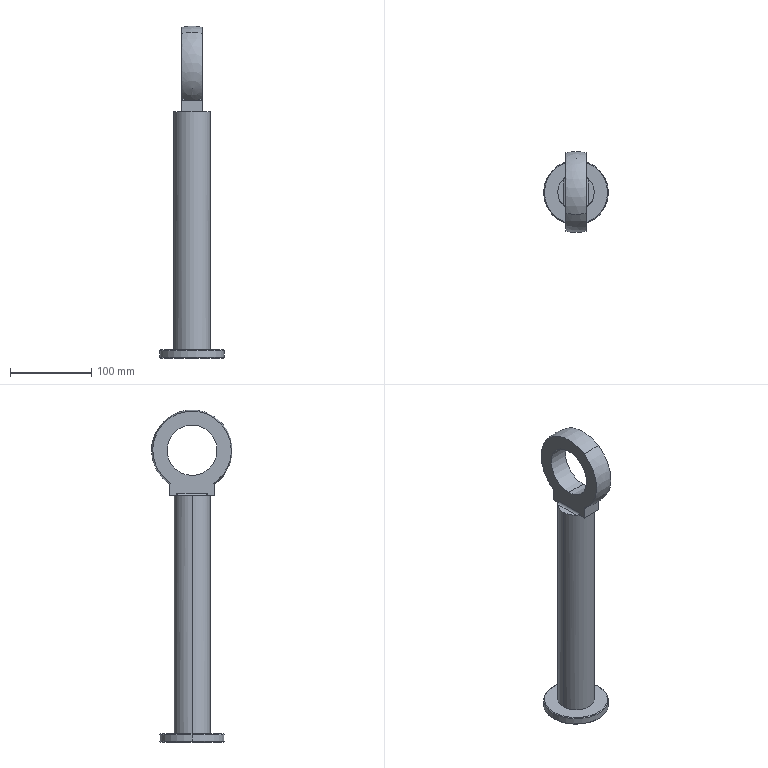Part | SolidWorks | features ICE 3, Chamfer 1, Extrusion 1, Fillet 1, RevCut 1 | 1 solid | 26 faces | box 80 x 100 x 410 mm | volume 647180 mm3 | plane 12 | cylinder 8 | cone 4 | sphere 2 | commonest cylinder face diameters 6 x2 45 x2 62 x2 80 x2
STEP:
#1=CARTESIAN_POINT('',(-12.5,0.,391.));
#2=VERTEX_POINT('',#1);
#3=CARTESIAN_POINT('',(-12.5,0.,329.));
#4=VERTEX_POINT('',#3);
#5=CARTESIAN_POINT('',(-12.5,0.,360.));
#6=DIRECTION('',(1.,0.,0.));
#7=DIRECTION('',(0.,0.,-1.));
#8=AXIS2_PLACEMENT_3D('',#5,#6,#7);
#9=CIRCLE('',#8,31.);
#10=EDGE_CURVE('',#2,#4,#9,.T.);
#11=ORIENTED_EDGE('',*,*,#10,.F.);
#12=CARTESIAN_POINT('',(12.5,0.,391.));
#13=VERTEX_POINT('',#12);
#14=CARTESIAN_POINT('',(-40.,0.,391.));
#15=DIRECTION('',(1.,0.,0.));
#16=VECTOR('',#15,1000.);
#17=LINE('',#14,#16);
#18=EDGE_CURVE('',#2,#13,#17,.T.);
#19=ORIENTED_EDGE('',*,*,#18,.T.);
#20=CARTESIAN_POINT('',(12.5,0.,329.));
#21=VERTEX_POINT('',#20);
#22=CARTESIAN_POINT('',(12.5,0.,360.));
#23=DIRECTION('',(1.,0.,0.));
#24=DIRECTION('',(0.,0.,-1.));
#25=AXIS2_PLACEMENT_3D('',#22,#23,#24);
#26=CIRCLE('',#25,31.);
#27=EDGE_CURVE('',#13,#21,#26,.T.);
#28=ORIENTED_EDGE('',*,*,#27,.T.);
#29=CARTESIAN_POINT('',(-40.,0.,329.));
#30=DIRECTION('',(1.,0.,0.));
#31=VECTOR('',#30,1000.);
#32=LINE('',#29,#31);
#33=EDGE_CURVE('',#4,#21,#32,.T.);
#34=ORIENTED_EDGE('',*,*,#33,.F.);
#35=EDGE_LOOP('',(#11,#19,#28,#34));
#36=FACE_OUTER_BOUND('',#35,.T.);
#37=CARTESIAN_POINT('',(-40.,0.,360.));
#38=DIRECTION('',(1.,0.,0.));
#39=DIRECTION('',(0.,0.,-1.));
#40=AXIS2_PLACEMENT_3D('',#37,#38,#39);
#41=CYLINDRICAL_SURFACE('',#40,31.);
#42=ADVANCED_FACE('',(#36),#41,.F.);
#43=CARTESIAN_POINT('',(-12.5,26.615,319.56));
#44=VERTEX_POINT('',#43);
#45=CARTESIAN_POINT('',(-12.5,-26.615,400.44));
#46=VERTEX_POINT('',#45);
#47=CARTESIAN_POINT('',(-12.5,0.,360.));
#48=DIRECTION('',(1.,0.,0.));
#49=DIRECTION('',(0.,0.,-1.));
#50=AXIS2_PLACEMENT_3D('',#47,#48,#49);
#51=CIRCLE('',#50,48.412);
#52=EDGE_CURVE('',#44,#46,#51,.T.);
#53=ORIENTED_EDGE('',*,*,#52,.T.);
#54=CARTESIAN_POINT('',(12.5,-26.615,400.44));
#55=VERTEX_POINT('',#54);
#56=CARTESIAN_POINT('',(0.,0.,360.));
#57=DIRECTION('',(0.,0.8353,0.5498));
#58=DIRECTION('',(0.,-0.5498,0.8353));
#59=AXIS2_PLACEMENT_3D('',#56,#57,#58);
#60=CIRCLE('',#59,50.);
#61=EDGE_CURVE('',#46,#55,#60,.T.);
#62=ORIENTED_EDGE('',*,*,#61,.T.);
#63=CARTESIAN_POINT('',(12.5,26.615,319.56));
#64=VERTEX_POINT('',#63);
#65=CARTESIAN_POINT('',(12.5,0.,360.));
#66=DIRECTION('',(1.,0.,0.));
#67=DIRECTION('',(0.,0.,-1.));
#68=AXIS2_PLACEMENT_3D('',#65,#66,#67);
#69=CIRCLE('',#68,48.412);
#70=EDGE_CURVE('',#64,#55,#69,.T.);
#71=ORIENTED_EDGE('',*,*,#70,.F.);
#72=CARTESIAN_POINT('',(0.,0.,360.));
#73=DIRECTION('',(0.,0.8353,0.5498));
#74=DIRECTION('',(0.,0.5498,-0.8353));
#75=AXIS2_PLACEMENT_3D('',#72,#73,#74);
#76=CIRCLE('',#75,50.);
#77=EDGE_CURVE('',#64,#44,#76,.T.);
#78=ORIENTED_EDGE('',*,*,#77,.T.);
#79=EDGE_LOOP('',(#53,#62,#71,#78));
#80=FACE_OUTER_BOUND('',#79,.T.);
#81=CARTESIAN_POINT('',(0.,0.,360.));
#82=DIRECTION('',(0.,0.8353,0.5498));
#83=DIRECTION('',(0.,0.5498,-0.8353));
#84=AXIS2_PLACEMENT_3D('',#81,#82,#83);
#85=SPHERICAL_SURFACE('',#84,50.);
#86=ADVANCED_FACE('',(#80),#85,.T.);
#87=CARTESIAN_POINT('',(39.,0.,10.));
#88=VERTEX_POINT('',#87);
#89=CARTESIAN_POINT('',(-39.,0.,10.));
#90=VERTEX_POINT('',#89);
#91=CARTESIAN_POINT('',(0.,0.,10.));
#92=DIRECTION('',(0.,0.,1.));
#93=DIRECTION('',(1.,0.,0.));
#94=AXIS2_PLACEMENT_3D('',#91,#92,#93);
#95=CIRCLE('',#94,39.);
#96=EDGE_CURVE('',#88,#90,#95,.T.);
#97=ORIENTED_EDGE('',*,*,#96,.F.);
#98=CARTESIAN_POINT('',(40.,0.,9.));
#99=VERTEX_POINT('',#98);
#100=CARTESIAN_POINT('',(39.,0.,10.));
#101=DIRECTION('',(0.7071,0.,-0.7071));
#102=VECTOR('',#101,1000.);
#103=LINE('',#100,#102);
#104=EDGE_CURVE('',#88,#99,#103,.T.);
#105=ORIENTED_EDGE('',*,*,#104,.T.);
#106=CARTESIAN_POINT('',(-40.,0.,9.));
#107=VERTEX_POINT('',#106);
#108=CARTESIAN_POINT('',(0.,0.,9.));
#109=DIRECTION('',(0.,0.,-1.));
#110=DIRECTION('',(1.,0.,0.));
#111=AXIS2_PLACEMENT_3D('',#108,#109,#110);
#112=CIRCLE('',#111,40.);
#113=EDGE_CURVE('',#107,#99,#112,.T.);
#114=ORIENTED_EDGE('',*,*,#113,.F.);
#115=CARTESIAN_POINT('',(-39.,0.,10.));
#116=DIRECTION('',(-0.7071,0.,-0.7071));
#117=VECTOR('',#116,1000.);
#118=LINE('',#115,#117);
#119=EDGE_CURVE('',#90,#107,#118,.T.);
#120=ORIENTED_EDGE('',*,*,#119,.F.);
#121=EDGE_LOOP('',(#97,#105,#114,#120));
#122=FACE_OUTER_BOUND('',#121,.T.);
#123=CARTESIAN_POINT('',(0.,0.,10.));
#124=DIRECTION('',(0.,0.,-1.));
#125=DIRECTION('',(-1.,0.,0.));
#126=AXIS2_PLACEMENT_3D('',#123,#124,#125);
#127=CONICAL_SURFACE('',#126,39.,0.7854);
#128=ADVANCED_FACE('',(#122),#127,.T.);
#129=CARTESIAN_POINT('',(-39.,0.,0.));
#130=VERTEX_POINT('',#129);
#131=CARTESIAN_POINT('',(39.,0.,0.));
#132=VERTEX_POINT('',#131);
#133=CARTESIAN_POINT('',(0.,0.,0.));
#134=DIRECTION('',(0.,0.,-1.));
#135=DIRECTION('',(1.,0.,0.));
#136=AXIS2_PLACEMENT_3D('',#133,#134,#135);
#137=CIRCLE('',#136,39.);
#138=EDGE_CURVE('',#130,#132,#137,.T.);
#139=ORIENTED_EDGE('',*,*,#138,.F.);
#140=CARTESIAN_POINT('',(-40.,0.,1.));
#141=VERTEX_POINT('',#140);
#142=CARTESIAN_POINT('',(-40.,0.,1.));
#143=DIRECTION('',(-0.7071,0.,0.7071));
#144=VECTOR('',#143,1000.);
#145=LINE('',#142,#144);
#146=EDGE_CURVE('',#130,#141,#145,.T.);
#147=ORIENTED_EDGE('',*,*,#146,.T.);
#148=CARTESIAN_POINT('',(40.,0.,1.));
#149=VERTEX_POINT('',#148);
#150=CARTESIAN_POINT('',(0.,0.,1.));
#151=DIRECTION('',(0.,0.,1.));
#152=DIRECTION('',(1.,0.,0.));
#153=AXIS2_PLACEMENT_3D('',#150,#151,#152);
#154=CIRCLE('',#153,40.);
#155=EDGE_CURVE('',#149,#141,#154,.T.);
#156=ORIENTED_EDGE('',*,*,#155,.F.);
#157=CARTESIAN_POINT('',(40.,0.,1.));
#158=DIRECTION('',(0.7071,0.,0.7071));
#159=VECTOR('',#158,1000.);
#160=LINE('',#157,#159);
#161=EDGE_CURVE('',#132,#149,#160,.T.);
#162=ORIENTED_EDGE('',*,*,#161,.F.);
#163=EDGE_LOOP('',(#139,#147,#156,#162));
#164=FACE_OUTER_BOUND('',#163,.T.);
#165=CARTESIAN_POINT('',(0.,0.,1.));
#166=DIRECTION('',(0.,0.,1.));
#167=DIRECTION('',(1.,0.,0.));
#168=AXIS2_PLACEMENT_3D('',#165,#166,#167);
#169=CONICAL_SURFACE('',#168,40.,0.7854);
#170=ADVANCED_FACE('',(#164),#169,.T.);
#171=CARTESIAN_POINT('',(22.5,0.,304.));
#172=VERTEX_POINT('',#171);
#173=CARTESIAN_POINT('',(15.5,16.31,304.));
#174=VERTEX_POINT('',#173);
#175=CARTESIAN_POINT('',(0.,0.,304.));
#176=DIRECTION('',(0.,0.,1.));
#177=DIRECTION('',(1.,0.,0.));
#178=AXIS2_PLACEMENT_3D('',#175,#176,#177);
#179=CIRCLE('',#178,22.5);
#180=EDGE_CURVE('',#172,#174,#179,.T.);
#181=ORIENTED_EDGE('',*,*,#180,.F.);
#182=CARTESIAN_POINT('',(22.5,0.,10.));
#183=VERTEX_POINT('',#182);
#184=CARTESIAN_POINT('',(22.5,0.,304.));
#185=DIRECTION('',(0.,0.,-1.));
#186=VECTOR('',#185,1000.);
#187=LINE('',#184,#186);
#188=EDGE_CURVE('',#172,#183,#187,.T.);
#189=ORIENTED_EDGE('',*,*,#188,.T.);
#190=CARTESIAN_POINT('',(-22.5,0.,10.));
#191=VERTEX_POINT('',#190);
#192=CARTESIAN_POINT('',(0.,0.,10.));
#193=DIRECTION('',(0.,0.,1.));
#194=DIRECTION('',(1.,0.,0.));
#195=AXIS2_PLACEMENT_3D('',#192,#193,#194);
#196=CIRCLE('',#195,22.5);
#197=EDGE_CURVE('',#183,#191,#196,.T.);
#198=ORIENTED_EDGE('',*,*,#197,.T.);
#199=CARTESIAN_POINT('',(-22.5,0.,304.));
#200=VERTEX_POINT('',#199);
#201=CARTESIAN_POINT('',(-22.5,0.,304.));
#202=DIRECTION('',(0.,0.,-1.));
#203=VECTOR('',#202,1000.);
#204=LINE('',#201,#203);
#205=EDGE_CURVE('',#200,#191,#204,.T.);
#206=ORIENTED_EDGE('',*,*,#205,.F.);
#207=CARTESIAN_POINT('',(-15.5,16.31,304.));
#208=VERTEX_POINT('',#207);
#209=CARTESIAN_POINT('',(0.,0.,304.));
#210=DIRECTION('',(0.,0.,1.));
#211=DIRECTION('',(1.,0.,0.));
#212=AXIS2_PLACEMENT_3D('',#209,#210,#211);
#213=CIRCLE('',#212,22.5);
#214=EDGE_CURVE('',#208,#200,#213,.T.);
#215=ORIENTED_EDGE('',*,*,#214,.F.);
#216=CARTESIAN_POINT('',(-12.5,18.708,307.));
#217=VERTEX_POINT('',#216);
#218=CARTESIAN_POINT('',(-15.5,16.31,304.));
#219=CARTESIAN_POINT('',(-15.171,16.622,304.));
#220=CARTESIAN_POINT('',(-14.838,16.92,304.053));
#221=CARTESIAN_POINT('',(-14.337,17.342,304.229));
#222=CARTESIAN_POINT('',(-14.17,17.479,304.305));
#223=CARTESIAN_POINT('',(-13.849,17.734,304.488));
#224=CARTESIAN_POINT('',(-13.693,17.855,304.597));
#225=CARTESIAN_POINT('',(-13.394,18.08,304.855));
#226=CARTESIAN_POINT('',(-13.254,18.183,305.001));
#227=CARTESIAN_POINT('',(-13.001,18.364,305.327));
#228=CARTESIAN_POINT('',(-12.887,18.444,305.511));
#229=CARTESIAN_POINT('',(-12.701,18.573,305.9));
#230=CARTESIAN_POINT('',(-12.627,18.623,306.106));
#231=CARTESIAN_POINT('',(-12.526,18.691,306.544));
#232=CARTESIAN_POINT('',(-12.5,18.708,306.771));
#233=CARTESIAN_POINT('',(-12.5,18.708,307.));
#234=B_SPLINE_CURVE_WITH_KNOTS('',3,(#218,#219,#220,#221,#222,#223,#224,#225,#226,#227,#228,#229,#230,#231,#232,#233),.UNSPECIFIED.,.F.,.F.,(4,2,2,2,2,2,2,4),(0.,0.001348,0.002022,0.002696,0.003369,0.004043,0.004717,0.005391),.UNSPECIFIED.);
#235=EDGE_CURVE('',#208,#217,#234,.T.);
#236=ORIENTED_EDGE('',*,*,#235,.T.);
#237=CARTESIAN_POINT('',(-12.5,18.708,304.));
#238=VERTEX_POINT('',#237);
#239=CARTESIAN_POINT('',(-12.5,18.708,304.));
#240=DIRECTION('',(0.,0.,1.));
#241=VECTOR('',#240,1000.);
#242=LINE('',#239,#241);
#243=EDGE_CURVE('',#238,#217,#242,.T.);
#244=ORIENTED_EDGE('',*,*,#243,.F.);
#245=CARTESIAN_POINT('',(12.5,18.708,304.));
#246=VERTEX_POINT('',#245);
#247=CARTESIAN_POINT('',(0.,0.,304.));
#248=DIRECTION('',(0.,0.,1.));
#249=DIRECTION('',(1.,0.,0.));
#250=AXIS2_PLACEMENT_3D('',#247,#248,#249);
#251=CIRCLE('',#250,22.5);
#252=EDGE_CURVE('',#246,#238,#251,.T.);
#253=ORIENTED_EDGE('',*,*,#252,.F.);
#254=CARTESIAN_POINT('',(12.5,18.708,307.));
#255=VERTEX_POINT('',#254);
#256=CARTESIAN_POINT('',(12.5,18.708,307.));
#257=DIRECTION('',(0.,0.,-1.));
#258=VECTOR('',#257,1000.);
#259=LINE('',#256,#258);
#260=EDGE_CURVE('',#255,#246,#259,.T.);
#261=ORIENTED_EDGE('',*,*,#260,.F.);
#262=CARTESIAN_POINT('',(12.5,18.708,307.));
#263=CARTESIAN_POINT('',(12.5,18.708,306.771));
#264=CARTESIAN_POINT('',(12.526,18.691,306.548));
#265=CARTESIAN_POINT('',(12.626,18.624,306.112));
#266=CARTESIAN_POINT('',(12.7,18.573,305.901));
#267=CARTESIAN_POINT('',(12.887,18.444,305.511));
#268=CARTESIAN_POINT('',(13.001,18.365,305.328));
#269=CARTESIAN_POINT('',(13.254,18.183,305.));
#270=CARTESIAN_POINT('',(13.394,18.08,304.854));
#271=CARTESIAN_POINT('',(13.693,17.854,304.597));
#272=CARTESIAN_POINT('',(13.85,17.733,304.488));
#273=CARTESIAN_POINT('',(14.173,17.477,304.303));
#274=CARTESIAN_POINT('',(14.34,17.34,304.228));
#275=CARTESIAN_POINT('',(14.839,16.919,304.053));
#276=CARTESIAN_POINT('',(15.171,16.622,304.));
#277=CARTESIAN_POINT('',(15.5,16.31,304.));
#278=B_SPLINE_CURVE_WITH_KNOTS('',3,(#262,#263,#264,#265,#266,#267,#268,#269,#270,#271,#272,#273,#274,#275,#276,#277),.UNSPECIFIED.,.F.,.F.,(4,2,2,2,2,2,2,4),(0.,0.0006752,0.00135,0.002026,0.002701,0.003376,0.004051,0.005402),.UNSPECIFIED.);
#279=EDGE_CURVE('',#255,#174,#278,.T.);
#280=ORIENTED_EDGE('',*,*,#279,.T.);
#281=EDGE_LOOP('',(#181,#189,#198,#206,#215,#236,#244,#253,#261,#280));
#282=FACE_OUTER_BOUND('',#281,.T.);
#283=CARTESIAN_POINT('',(0.,0.,304.));
#284=DIRECTION('',(0.,0.,-1.));
#285=DIRECTION('',(-1.,0.,0.));
#286=AXIS2_PLACEMENT_3D('',#283,#284,#285);
#287=CYLINDRICAL_SURFACE('',#286,22.5);
#288=ADVANCED_FACE('',(#282),#287,.T.);
#289=ORIENTED_EDGE('',*,*,#113,.T.);
#290=CARTESIAN_POINT('',(40.,0.,10.));
#291=DIRECTION('',(0.,0.,-1.));
#292=VECTOR('',#291,1000.);
#293=LINE('',#290,#292);
#294=EDGE_CURVE('',#99,#149,#293,.T.);
#295=ORIENTED_EDGE('',*,*,#294,.T.);
#296=ORIENTED_EDGE('',*,*,#155,.T.);
#297=CARTESIAN_POINT('',(-40.,0.,10.));
#298=DIRECTION('',(0.,0.,-1.));
#299=VECTOR('',#298,1000.);
#300=LINE('',#297,#299);
#301=EDGE_CURVE('',#107,#141,#300,.T.);
#302=ORIENTED_EDGE('',*,*,#301,.F.);
#303=EDGE_LOOP('',(#289,#295,#296,#302));
#304=FACE_OUTER_BOUND('',#303,.T.);
#305=CARTESIAN_POINT('',(0.,0.,10.));
#306=DIRECTION('',(0.,0.,-1.));
#307=DIRECTION('',(-1.,0.,0.));
#308=AXIS2_PLACEMENT_3D('',#305,#306,#307);
#309=CYLINDRICAL_SURFACE('',#308,40.);
#310=ADVANCED_FACE('',(#304),#309,.T.);
#311=CARTESIAN_POINT('',(-12.5,-27.5,318.215));
#312=VERTEX_POINT('',#311);
#313=CARTESIAN_POINT('',(12.5,-27.5,318.215));
#314=VERTEX_POINT('',#313);
#315=CARTESIAN_POINT('',(12.5,-27.5,318.215));
#316=DIRECTION('',(1.,0.,0.));
#317=VECTOR('',#316,1000.);
#318=LINE('',#315,#317);
#319=EDGE_CURVE('',#312,#314,#318,.T.);
#320=ORIENTED_EDGE('',*,*,#319,.F.);
#321=CARTESIAN_POINT('',(-12.5,-27.5,304.));
#322=VERTEX_POINT('',#321);
#323=CARTESIAN_POINT('',(-12.5,-27.5,304.));
#324=DIRECTION('',(0.,0.,-1.));
#325=VECTOR('',#324,1000.);
#326=LINE('',#323,#325);
#327=EDGE_CURVE('',#312,#322,#326,.T.);
#328=ORIENTED_EDGE('',*,*,#327,.T.);
#329=CARTESIAN_POINT('',(12.5,-27.5,304.));
#330=VERTEX_POINT('',#329);
#331=CARTESIAN_POINT('',(12.5,-27.5,304.));
#332=DIRECTION('',(-1.,0.,0.));
#333=VECTOR('',#332,1000.);
#334=LINE('',#331,#333);
#335=EDGE_CURVE('',#330,#322,#334,.T.);
#336=ORIENTED_EDGE('',*,*,#335,.F.);
#337=CARTESIAN_POINT('',(12.5,-27.5,304.));
#338=DIRECTION('',(0.,0.,-1.));
#339=VECTOR('',#338,1000.);
#340=LINE('',#337,#339);
#341=EDGE_CURVE('',#314,#330,#340,.T.);
#342=ORIENTED_EDGE('',*,*,#341,.F.);
#343=EDGE_LOOP('',(#320,#328,#336,#342));
#344=FACE_OUTER_BOUND('',#343,.T.);
#345=CARTESIAN_POINT('',(12.5,-27.5,304.));
#346=DIRECTION('',(0.,1.,0.));
#347=DIRECTION('',(0.,0.,1.));
#348=AXIS2_PLACEMENT_3D('',#345,#346,#347);
#349=PLANE('',#348);
#350=ADVANCED_FACE('',(#344),#349,.F.);
#351=ORIENTED_EDGE('',*,*,#214,.T.);
#352=CARTESIAN_POINT('',(-15.5,-16.31,304.));
#353=VERTEX_POINT('',#352);
#354=CARTESIAN_POINT('',(0.,0.,304.));
#355=DIRECTION('',(0.,0.,1.));
#356=DIRECTION('',(1.,0.,0.));
#357=AXIS2_PLACEMENT_3D('',#354,#355,#356);
#358=CIRCLE('',#357,22.5);
#359=EDGE_CURVE('',#200,#353,#358,.T.);
#360=ORIENTED_EDGE('',*,*,#359,.T.);
#361=CARTESIAN_POINT('',(-15.5,0.,304.));
#362=DIRECTION('',(0.,1.,0.));
#363=VECTOR('',#362,1000.);
#364=LINE('',#361,#363);
#365=EDGE_CURVE('',#353,#208,#364,.T.);
#366=ORIENTED_EDGE('',*,*,#365,.T.);
#367=EDGE_LOOP('',(#351,#360,#366));
#368=FACE_OUTER_BOUND('',#367,.T.);
#369=CARTESIAN_POINT('',(0.,0.,304.));
#370=DIRECTION('',(0.,0.,1.));
#371=DIRECTION('',(1.,0.,0.));
#372=AXIS2_PLACEMENT_3D('',#369,#370,#371);
#373=PLANE('',#372);
#374=ADVANCED_FACE('',(#368),#373,.T.);
#375=CARTESIAN_POINT('',(0.,0.,10.));
#376=DIRECTION('',(0.,0.,1.));
#377=DIRECTION('',(1.,0.,0.));
#378=AXIS2_PLACEMENT_3D('',#375,#376,#377);
#379=CIRCLE('',#378,39.);
#380=EDGE_CURVE('',#90,#88,#379,.T.);
#381=ORIENTED_EDGE('',*,*,#380,.T.);
#382=ORIENTED_EDGE('',*,*,#96,.T.);
#383=EDGE_LOOP('',(#381,#382));
#384=FACE_OUTER_BOUND('',#383,.T.);
#385=CARTESIAN_POINT('',(0.,0.,10.));
#386=DIRECTION('',(0.,0.,1.));
#387=DIRECTION('',(1.,0.,0.));
#388=AXIS2_PLACEMENT_3D('',#385,#386,#387);
#389=CIRCLE('',#388,22.5);
#390=EDGE_CURVE('',#191,#183,#389,.T.);
#391=ORIENTED_EDGE('',*,*,#390,.F.);
#392=ORIENTED_EDGE('',*,*,#197,.F.);
#393=EDGE_LOOP('',(#391,#392));
#394=FACE_BOUND('',#393,.T.);
#395=CARTESIAN_POINT('',(0.,0.,10.));
#396=DIRECTION('',(0.,0.,1.));
#397=DIRECTION('',(1.,0.,0.));
#398=AXIS2_PLACEMENT_3D('',#395,#396,#397);
#399=PLANE('',#398);
#400=ADVANCED_FACE('',(#384,#394),#399,.T.);
#401=ORIENTED_EDGE('',*,*,#294,.F.);
#402=CARTESIAN_POINT('',(0.,0.,9.));
#403=DIRECTION('',(0.,0.,-1.));
#404=DIRECTION('',(1.,0.,0.));
#405=AXIS2_PLACEMENT_3D('',#402,#403,#404);
#406=CIRCLE('',#405,40.);
#407=EDGE_CURVE('',#99,#107,#406,.T.);
#408=ORIENTED_EDGE('',*,*,#407,.T.);
#409=ORIENTED_EDGE('',*,*,#301,.T.);
#410=CARTESIAN_POINT('',(0.,0.,1.));
#411=DIRECTION('',(0.,0.,1.));
#412=DIRECTION('',(1.,0.,0.));
#413=AXIS2_PLACEMENT_3D('',#410,#411,#412);
#414=CIRCLE('',#413,40.);
#415=EDGE_CURVE('',#141,#149,#414,.T.);
#416=ORIENTED_EDGE('',*,*,#415,.T.);
#417=EDGE_LOOP('',(#401,#408,#409,#416));
#418=FACE_OUTER_BOUND('',#417,.T.);
#419=CARTESIAN_POINT('',(0.,0.,10.));
#420=DIRECTION('',(0.,0.,-1.));
#421=DIRECTION('',(-1.,0.,0.));
#422=AXIS2_PLACEMENT_3D('',#419,#420,#421);
#423=CYLINDRICAL_SURFACE('',#422,40.);
#424=ADVANCED_FACE('',(#418),#423,.T.);
#425=CARTESIAN_POINT('',(0.,0.,0.));
#426=DIRECTION('',(0.,0.,-1.));
#427=DIRECTION('',(1.,0.,0.));
#428=AXIS2_PLACEMENT_3D('',#425,#426,#427);
#429=CIRCLE('',#428,39.);
#430=EDGE_CURVE('',#132,#130,#429,.T.);
#431=ORIENTED_EDGE('',*,*,#430,.T.);
#432=ORIENTED_EDGE('',*,*,#138,.T.);
#433=EDGE_LOOP('',(#431,#432));
#434=FACE_OUTER_BOUND('',#433,.T.);
#435=CARTESIAN_POINT('',(0.,0.,0.));
#436=DIRECTION('',(0.,0.,1.));
#437=DIRECTION('',(1.,0.,0.));
#438=AXIS2_PLACEMENT_3D('',#435,#436,#437);
#439=PLANE('',#438);
#440=ADVANCED_FACE('',(#434),#439,.F.);
#441=ORIENTED_EDGE('',*,*,#188,.F.);
#442=CARTESIAN_POINT('',(15.5,-16.31,304.));
#443=VERTEX_POINT('',#442);
#444=CARTESIAN_POINT('',(0.,0.,304.));
#445=DIRECTION('',(0.,0.,1.));
#446=DIRECTION('',(1.,0.,0.));
#447=AXIS2_PLACEMENT_3D('',#444,#445,#446);
#448=CIRCLE('',#447,22.5);
#449=EDGE_CURVE('',#443,#172,#448,.T.);
#450=ORIENTED_EDGE('',*,*,#449,.F.);
#451=CARTESIAN_POINT('',(12.5,-18.708,307.));
#452=VERTEX_POINT('',#451);
#453=CARTESIAN_POINT('',(15.5,-16.31,304.));
#454=CARTESIAN_POINT('',(15.171,-16.622,304.));
#455=CARTESIAN_POINT('',(14.838,-16.92,304.053));
#456=CARTESIAN_POINT('',(14.337,-17.342,304.229));
#457=CARTESIAN_POINT('',(14.17,-17.479,304.305));
#458=CARTESIAN_POINT('',(13.849,-17.734,304.488));
#459=CARTESIAN_POINT('',(13.693,-17.855,304.597));
#460=CARTESIAN_POINT('',(13.394,-18.08,304.855));
#461=CARTESIAN_POINT('',(13.254,-18.183,305.001));
#462=CARTESIAN_POINT('',(13.001,-18.364,305.327));
#463=CARTESIAN_POINT('',(12.887,-18.444,305.511));
#464=CARTESIAN_POINT('',(12.701,-18.573,305.9));
#465=CARTESIAN_POINT('',(12.627,-18.623,306.106));
#466=CARTESIAN_POINT('',(12.526,-18.691,306.544));
#467=CARTESIAN_POINT('',(12.5,-18.708,306.771));
#468=CARTESIAN_POINT('',(12.5,-18.708,307.));
#469=B_SPLINE_CURVE_WITH_KNOTS('',3,(#453,#454,#455,#456,#457,#458,#459,#460,#461,#462,#463,#464,#465,#466,#467,#468),.UNSPECIFIED.,.F.,.F.,(4,2,2,2,2,2,2,4),(0.,0.001348,0.002022,0.002696,0.003369,0.004043,0.004717,0.005391),.UNSPECIFIED.);
#470=EDGE_CURVE('',#443,#452,#469,.T.);
#471=ORIENTED_EDGE('',*,*,#470,.T.);
#472=CARTESIAN_POINT('',(12.5,-18.708,304.));
#473=VERTEX_POINT('',#472);
#474=CARTESIAN_POINT('',(12.5,-18.708,304.));
#475=DIRECTION('',(0.,0.,1.));
#476=VECTOR('',#475,1000.);
#477=LINE('',#474,#476);
#478=EDGE_CURVE('',#473,#452,#477,.T.);
#479=ORIENTED_EDGE('',*,*,#478,.F.);
#480=CARTESIAN_POINT('',(-12.5,-18.708,304.));
#481=VERTEX_POINT('',#480);
#482=CARTESIAN_POINT('',(0.,0.,304.));
#483=DIRECTION('',(0.,0.,1.));
#484=DIRECTION('',(1.,0.,0.));
#485=AXIS2_PLACEMENT_3D('',#482,#483,#484);
#486=CIRCLE('',#485,22.5);
#487=EDGE_CURVE('',#481,#473,#486,.T.);
#488=ORIENTED_EDGE('',*,*,#487,.F.);
#489=CARTESIAN_POINT('',(-12.5,-18.708,307.));
#490=VERTEX_POINT('',#489);
#491=CARTESIAN_POINT('',(-12.5,-18.708,307.));
#492=DIRECTION('',(0.,0.,-1.));
#493=VECTOR('',#492,1000.);
#494=LINE('',#491,#493);
#495=EDGE_CURVE('',#490,#481,#494,.T.);
#496=ORIENTED_EDGE('',*,*,#495,.F.);
#497=CARTESIAN_POINT('',(-12.5,-18.708,307.));
#498=CARTESIAN_POINT('',(-12.5,-18.708,306.771));
#499=CARTESIAN_POINT('',(-12.526,-18.691,306.548));
#500=CARTESIAN_POINT('',(-12.626,-18.624,306.112));
#501=CARTESIAN_POINT('',(-12.7,-18.573,305.901));
#502=CARTESIAN_POINT('',(-12.887,-18.444,305.511));
#503=CARTESIAN_POINT('',(-13.001,-18.365,305.328));
#504=CARTESIAN_POINT('',(-13.254,-18.183,305.));
#505=CARTESIAN_POINT('',(-13.394,-18.08,304.854));
#506=CARTESIAN_POINT('',(-13.693,-17.854,304.597));
#507=CARTESIAN_POINT('',(-13.85,-17.733,304.488));
#508=CARTESIAN_POINT('',(-14.173,-17.477,304.303));
#509=CARTESIAN_POINT('',(-14.34,-17.34,304.228));
#510=CARTESIAN_POINT('',(-14.839,-16.919,304.053));
#511=CARTESIAN_POINT('',(-15.171,-16.622,304.));
#512=CARTESIAN_POINT('',(-15.5,-16.31,304.));
#513=B_SPLINE_CURVE_WITH_KNOTS('',3,(#497,#498,#499,#500,#501,#502,#503,#504,#505,#506,#507,#508,#509,#510,#511,#512),.UNSPECIFIED.,.F.,.F.,(4,2,2,2,2,2,2,4),(0.,0.0006752,0.00135,0.002026,0.002701,0.003376,0.004051,0.005402),.UNSPECIFIED.);
#514=EDGE_CURVE('',#490,#353,#513,.T.);
#515=ORIENTED_EDGE('',*,*,#514,.T.);
#516=ORIENTED_EDGE('',*,*,#359,.F.);
#517=ORIENTED_EDGE('',*,*,#205,.T.);
#518=ORIENTED_EDGE('',*,*,#390,.T.);
#519=EDGE_LOOP('',(#441,#450,#471,#479,#488,#496,#515,#516,#517,#518));
#520=FACE_OUTER_BOUND('',#519,.T.);
#521=CARTESIAN_POINT('',(0.,0.,304.));
#522=DIRECTION('',(0.,0.,-1.));
#523=DIRECTION('',(-1.,0.,0.));
#524=AXIS2_PLACEMENT_3D('',#521,#522,#523);
#525=CYLINDRICAL_SURFACE('',#524,22.5);
#526=ADVANCED_FACE('',(#520),#525,.T.);
#527=ORIENTED_EDGE('',*,*,#449,.T.);
#528=ORIENTED_EDGE('',*,*,#180,.T.);
#529=CARTESIAN_POINT('',(15.5,-18.708,304.));
#530=DIRECTION('',(0.,-1.,0.));
#531=VECTOR('',#530,1000.);
#532=LINE('',#529,#531);
#533=EDGE_CURVE('',#174,#443,#532,.T.);
#534=ORIENTED_EDGE('',*,*,#533,.T.);
#535=EDGE_LOOP('',(#527,#528,#534));
#536=FACE_OUTER_BOUND('',#535,.T.);
#537=CARTESIAN_POINT('',(0.,0.,304.));
#538=DIRECTION('',(0.,0.,1.));
#539=DIRECTION('',(1.,0.,0.));
#540=AXIS2_PLACEMENT_3D('',#537,#538,#539);
#541=PLANE('',#540);
#542=ADVANCED_FACE('',(#536),#541,.T.);
#543=ORIENTED_EDGE('',*,*,#146,.F.);
#544=ORIENTED_EDGE('',*,*,#430,.F.);
#545=ORIENTED_EDGE('',*,*,#161,.T.);
#546=ORIENTED_EDGE('',*,*,#415,.F.);
#547=EDGE_LOOP('',(#543,#544,#545,#546));
#548=FACE_OUTER_BOUND('',#547,.T.);
#549=CARTESIAN_POINT('',(0.,0.,1.));
#550=DIRECTION('',(0.,0.,1.));
#551=DIRECTION('',(1.,0.,0.));
#552=AXIS2_PLACEMENT_3D('',#549,#550,#551);
#553=CONICAL_SURFACE('',#552,40.,0.7854);
#554=ADVANCED_FACE('',(#548),#553,.T.);
#555=ORIENTED_EDGE('',*,*,#104,.F.);
#556=ORIENTED_EDGE('',*,*,#380,.F.);
#557=ORIENTED_EDGE('',*,*,#119,.T.);
#558=ORIENTED_EDGE('',*,*,#407,.F.);
#559=EDGE_LOOP('',(#555,#556,#557,#558));
#560=FACE_OUTER_BOUND('',#559,.T.);
#561=CARTESIAN_POINT('',(0.,0.,10.));
#562=DIRECTION('',(0.,0.,-1.));
#563=DIRECTION('',(-1.,0.,0.));
#564=AXIS2_PLACEMENT_3D('',#561,#562,#563);
#565=CONICAL_SURFACE('',#564,39.,0.7854);
#566=ADVANCED_FACE('',(#560),#565,.T.);
#567=CARTESIAN_POINT('',(12.5,27.5,304.));
#568=VERTEX_POINT('',#567);
#569=CARTESIAN_POINT('',(12.5,27.5,304.));
#570=DIRECTION('',(0.,1.,0.));
#571=VECTOR('',#570,1000.);
#572=LINE('',#569,#571);
#573=EDGE_CURVE('',#246,#568,#572,.T.);
#574=ORIENTED_EDGE('',*,*,#573,.F.);
#575=ORIENTED_EDGE('',*,*,#252,.T.);
#576=CARTESIAN_POINT('',(-12.5,27.5,304.));
#577=VERTEX_POINT('',#576);
#578=CARTESIAN_POINT('',(-12.5,27.5,304.));
#579=DIRECTION('',(0.,1.,0.));
#580=VECTOR('',#579,1000.);
#581=LINE('',#578,#580);
#582=EDGE_CURVE('',#238,#577,#581,.T.);
#583=ORIENTED_EDGE('',*,*,#582,.T.);
#584=CARTESIAN_POINT('',(12.5,27.5,304.));
#585=DIRECTION('',(-1.,0.,0.));
#586=VECTOR('',#585,1000.);
#587=LINE('',#584,#586);
#588=EDGE_CURVE('',#568,#577,#587,.T.);
#589=ORIENTED_EDGE('',*,*,#588,.F.);
#590=EDGE_LOOP('',(#574,#575,#583,#589));
#591=FACE_OUTER_BOUND('',#590,.T.);
#592=CARTESIAN_POINT('',(12.5,27.5,304.));
#593=DIRECTION('',(0.,0.,1.));
#594=DIRECTION('',(1.,0.,0.));
#595=AXIS2_PLACEMENT_3D('',#592,#593,#594);
#596=PLANE('',#595);
#597=ADVANCED_FACE('',(#591),#596,.F.);
#598=CARTESIAN_POINT('',(-12.5,27.5,304.));
#599=DIRECTION('',(0.,1.,0.));
#600=VECTOR('',#599,1000.);
#601=LINE('',#598,#600);
#602=EDGE_CURVE('',#322,#481,#601,.T.);
#603=ORIENTED_EDGE('',*,*,#602,.T.);
#604=ORIENTED_EDGE('',*,*,#487,.T.);
#605=CARTESIAN_POINT('',(12.5,27.5,304.));
#606=DIRECTION('',(0.,1.,0.));
#607=VECTOR('',#606,1000.);
#608=LINE('',#605,#607);
#609=EDGE_CURVE('',#330,#473,#608,.T.);
#610=ORIENTED_EDGE('',*,*,#609,.F.);
#611=ORIENTED_EDGE('',*,*,#335,.T.);
#612=EDGE_LOOP('',(#603,#604,#610,#611));
#613=FACE_OUTER_BOUND('',#612,.T.);
#614=CARTESIAN_POINT('',(12.5,27.5,304.));
#615=DIRECTION('',(0.,0.,1.));
#616=DIRECTION('',(1.,0.,0.));
#617=AXIS2_PLACEMENT_3D('',#614,#615,#616);
#618=PLANE('',#617);
#619=ADVANCED_FACE('',(#613),#618,.F.);
#620=CARTESIAN_POINT('',(12.5,0.,360.));
#621=DIRECTION('',(1.,0.,0.));
#622=DIRECTION('',(0.,0.,-1.));
#623=AXIS2_PLACEMENT_3D('',#620,#621,#622);
#624=CIRCLE('',#623,31.);
#625=EDGE_CURVE('',#21,#13,#624,.T.);
#626=ORIENTED_EDGE('',*,*,#625,.F.);
#627=ORIENTED_EDGE('',*,*,#27,.F.);
#628=EDGE_LOOP('',(#626,#627));
#629=FACE_BOUND('',#628,.T.);
#630=CARTESIAN_POINT('',(12.5,18.708,307.));
#631=DIRECTION('',(0.,1.,0.));
#632=VECTOR('',#631,1000.);
#633=LINE('',#630,#632);
#634=EDGE_CURVE('',#452,#255,#633,.T.);
#635=ORIENTED_EDGE('',*,*,#634,.T.);
#636=ORIENTED_EDGE('',*,*,#260,.T.);
#637=ORIENTED_EDGE('',*,*,#573,.T.);
#638=CARTESIAN_POINT('',(12.5,27.5,318.215));
#639=VERTEX_POINT('',#638);
#640=CARTESIAN_POINT('',(12.5,27.5,304.));
#641=DIRECTION('',(0.,0.,1.));
#642=VECTOR('',#641,1000.);
#643=LINE('',#640,#642);
#644=EDGE_CURVE('',#568,#639,#643,.T.);
#645=ORIENTED_EDGE('',*,*,#644,.T.);
#646=CARTESIAN_POINT('',(12.5,29.21,315.616));
#647=DIRECTION('',(0.,-0.5498,0.8353));
#648=VECTOR('',#647,1000.);
#649=LINE('',#646,#648);
#650=EDGE_CURVE('',#639,#64,#649,.T.);
#651=ORIENTED_EDGE('',*,*,#650,.T.);
#652=ORIENTED_EDGE('',*,*,#70,.T.);
#653=CARTESIAN_POINT('',(12.5,-26.615,319.56));
#654=VERTEX_POINT('',#653);
#655=CARTESIAN_POINT('',(12.5,0.,360.));
#656=DIRECTION('',(1.,0.,0.));
#657=DIRECTION('',(0.,0.,-1.));
#658=AXIS2_PLACEMENT_3D('',#655,#656,#657);
#659=CIRCLE('',#658,48.412);
#660=EDGE_CURVE('',#55,#654,#659,.T.);
#661=ORIENTED_EDGE('',*,*,#660,.T.);
#662=CARTESIAN_POINT('',(12.5,-29.21,315.616));
#663=DIRECTION('',(0.,0.5498,0.8353));
#664=VECTOR('',#663,1000.);
#665=LINE('',#662,#664);
#666=EDGE_CURVE('',#314,#654,#665,.T.);
#667=ORIENTED_EDGE('',*,*,#666,.F.);
#668=ORIENTED_EDGE('',*,*,#341,.T.);
#669=ORIENTED_EDGE('',*,*,#609,.T.);
#670=ORIENTED_EDGE('',*,*,#478,.T.);
#671=EDGE_LOOP('',(#635,#636,#637,#645,#651,#652,#661,#667,#668,#669,#670));
#672=FACE_OUTER_BOUND('',#671,.T.);
#673=CARTESIAN_POINT('',(12.5,0.,360.));
#674=DIRECTION('',(1.,0.,0.));
#675=DIRECTION('',(0.,0.,-1.));
#676=AXIS2_PLACEMENT_3D('',#673,#674,#675);
#677=PLANE('',#676);
#678=ADVANCED_FACE('',(#629,#672),#677,.T.);
#679=CARTESIAN_POINT('',(-12.5,0.,360.));
#680=DIRECTION('',(1.,0.,0.));
#681=DIRECTION('',(0.,0.,-1.));
#682=AXIS2_PLACEMENT_3D('',#679,#680,#681);
#683=CIRCLE('',#682,31.);
#684=EDGE_CURVE('',#4,#2,#683,.T.);
#685=ORIENTED_EDGE('',*,*,#684,.T.);
#686=ORIENTED_EDGE('',*,*,#10,.T.);
#687=EDGE_LOOP('',(#685,#686));
#688=FACE_BOUND('',#687,.T.);
#689=ORIENTED_EDGE('',*,*,#582,.F.);
#690=ORIENTED_EDGE('',*,*,#243,.T.);
#691=CARTESIAN_POINT('',(-12.5,0.,307.));
#692=DIRECTION('',(0.,-1.,0.));
#693=VECTOR('',#692,1000.);
#694=LINE('',#691,#693);
#695=EDGE_CURVE('',#217,#490,#694,.T.);
#696=ORIENTED_EDGE('',*,*,#695,.T.);
#697=ORIENTED_EDGE('',*,*,#495,.T.);
#698=ORIENTED_EDGE('',*,*,#602,.F.);
#699=ORIENTED_EDGE('',*,*,#327,.F.);
#700=CARTESIAN_POINT('',(-12.5,-26.615,319.56));
#701=VERTEX_POINT('',#700);
#702=CARTESIAN_POINT('',(-12.5,-26.615,319.56));
#703=DIRECTION('',(0.,-0.5498,-0.8353));
#704=VECTOR('',#703,1000.);
#705=LINE('',#702,#704);
#706=EDGE_CURVE('',#701,#312,#705,.T.);
#707=ORIENTED_EDGE('',*,*,#706,.F.);
#708=CARTESIAN_POINT('',(-12.5,0.,360.));
#709=DIRECTION('',(1.,0.,0.));
#710=DIRECTION('',(0.,0.,-1.));
#711=AXIS2_PLACEMENT_3D('',#708,#709,#710);
#712=CIRCLE('',#711,48.412);
#713=EDGE_CURVE('',#46,#701,#712,.T.);
#714=ORIENTED_EDGE('',*,*,#713,.F.);
#715=ORIENTED_EDGE('',*,*,#52,.F.);
#716=CARTESIAN_POINT('',(-12.5,27.5,318.215));
#717=VERTEX_POINT('',#716);
#718=CARTESIAN_POINT('',(-12.5,26.615,319.56));
#719=DIRECTION('',(0.,0.5498,-0.8353));
#720=VECTOR('',#719,1000.);
#721=LINE('',#718,#720);
#722=EDGE_CURVE('',#44,#717,#721,.T.);
#723=ORIENTED_EDGE('',*,*,#722,.T.);
#724=CARTESIAN_POINT('',(-12.5,27.5,304.));
#725=DIRECTION('',(0.,0.,1.));
#726=VECTOR('',#725,1000.);
#727=LINE('',#724,#726);
#728=EDGE_CURVE('',#577,#717,#727,.T.);
#729=ORIENTED_EDGE('',*,*,#728,.F.);
#730=EDGE_LOOP('',(#689,#690,#696,#697,#698,#699,#707,#714,#715,#723,#729));
#731=FACE_OUTER_BOUND('',#730,.T.);
#732=CARTESIAN_POINT('',(-12.5,0.,360.));
#733=DIRECTION('',(1.,0.,0.));
#734=DIRECTION('',(0.,0.,-1.));
#735=AXIS2_PLACEMENT_3D('',#732,#733,#734);
#736=PLANE('',#735);
#737=ADVANCED_FACE('',(#688,#731),#736,.F.);
#738=ORIENTED_EDGE('',*,*,#728,.T.);
#739=CARTESIAN_POINT('',(12.5,27.5,318.215));
#740=DIRECTION('',(1.,0.,0.));
#741=VECTOR('',#740,1000.);
#742=LINE('',#739,#741);
#743=EDGE_CURVE('',#717,#639,#742,.T.);
#744=ORIENTED_EDGE('',*,*,#743,.T.);
#745=ORIENTED_EDGE('',*,*,#644,.F.);
#746=ORIENTED_EDGE('',*,*,#588,.T.);
#747=EDGE_LOOP('',(#738,#744,#745,#746));
#748=FACE_OUTER_BOUND('',#747,.T.);
#749=CARTESIAN_POINT('',(12.5,27.5,304.));
#750=DIRECTION('',(0.,-1.,0.));
#751=DIRECTION('',(0.,0.,-1.));
#752=AXIS2_PLACEMENT_3D('',#749,#750,#751);
#753=PLANE('',#752);
#754=ADVANCED_FACE('',(#748),#753,.F.);
#755=ORIENTED_EDGE('',*,*,#722,.F.);
#756=ORIENTED_EDGE('',*,*,#77,.F.);
#757=ORIENTED_EDGE('',*,*,#650,.F.);
#758=ORIENTED_EDGE('',*,*,#743,.F.);
#759=EDGE_LOOP('',(#755,#756,#757,#758));
#760=FACE_OUTER_BOUND('',#759,.T.);
#761=CARTESIAN_POINT('',(0.,0.,360.));
#762=DIRECTION('',(0.,-0.8353,-0.5498));
#763=DIRECTION('',(0.,0.5498,-0.8353));
#764=AXIS2_PLACEMENT_3D('',#761,#762,#763);
#765=PLANE('',#764);
#766=ADVANCED_FACE('',(#760),#765,.F.);
#767=ORIENTED_EDGE('',*,*,#319,.T.);
#768=ORIENTED_EDGE('',*,*,#666,.T.);
#769=CARTESIAN_POINT('',(0.,0.,360.));
#770=DIRECTION('',(0.,0.8353,-0.5498));
#771=DIRECTION('',(0.,-0.5498,-0.8353));
#772=AXIS2_PLACEMENT_3D('',#769,#770,#771);
#773=CIRCLE('',#772,50.);
#774=EDGE_CURVE('',#654,#701,#773,.T.);
#775=ORIENTED_EDGE('',*,*,#774,.T.);
#776=ORIENTED_EDGE('',*,*,#706,.T.);
#777=EDGE_LOOP('',(#767,#768,#775,#776));
#778=FACE_OUTER_BOUND('',#777,.T.);
#779=CARTESIAN_POINT('',(0.,0.,360.));
#780=DIRECTION('',(0.,-0.8353,0.5498));
#781=DIRECTION('',(0.,-0.5498,-0.8353));
#782=AXIS2_PLACEMENT_3D('',#779,#780,#781);
#783=PLANE('',#782);
#784=ADVANCED_FACE('',(#778),#783,.T.);
#785=ORIENTED_EDGE('',*,*,#61,.F.);
#786=ORIENTED_EDGE('',*,*,#713,.T.);
#787=ORIENTED_EDGE('',*,*,#774,.F.);
#788=ORIENTED_EDGE('',*,*,#660,.F.);
#789=EDGE_LOOP('',(#785,#786,#787,#788));
#790=FACE_OUTER_BOUND('',#789,.T.);
#791=CARTESIAN_POINT('',(0.,0.,360.));
#792=DIRECTION('',(0.,0.8353,0.5498));
#793=DIRECTION('',(0.,0.5498,-0.8353));
#794=AXIS2_PLACEMENT_3D('',#791,#792,#793);
#795=SPHERICAL_SURFACE('',#794,50.);
#796=ADVANCED_FACE('',(#790),#795,.T.);
#797=ORIENTED_EDGE('',*,*,#514,.F.);
#798=ORIENTED_EDGE('',*,*,#695,.F.);
#799=ORIENTED_EDGE('',*,*,#235,.F.);
#800=ORIENTED_EDGE('',*,*,#365,.F.);
#801=EDGE_LOOP('',(#797,#798,#799,#800));
#802=FACE_OUTER_BOUND('',#801,.T.);
#803=CARTESIAN_POINT('',(-15.5,0.,307.));
#804=DIRECTION('',(0.,1.,0.));
#805=DIRECTION('',(0.,0.,1.));
#806=AXIS2_PLACEMENT_3D('',#803,#804,#805);
#807=CYLINDRICAL_SURFACE('',#806,3.);
#808=ADVANCED_FACE('',(#802),#807,.F.);
#809=ORIENTED_EDGE('',*,*,#470,.F.);
#810=ORIENTED_EDGE('',*,*,#533,.F.);
#811=ORIENTED_EDGE('',*,*,#279,.F.);
#812=ORIENTED_EDGE('',*,*,#634,.F.);
#813=EDGE_LOOP('',(#809,#810,#811,#812));
#814=FACE_OUTER_BOUND('',#813,.T.);
#815=CARTESIAN_POINT('',(15.5,0.,307.));
#816=DIRECTION('',(0.,-1.,0.));
#817=DIRECTION('',(0.,0.,-1.));
#818=AXIS2_PLACEMENT_3D('',#815,#816,#817);
#819=CYLINDRICAL_SURFACE('',#818,3.);
#820=ADVANCED_FACE('',(#814),#819,.F.);
#821=ORIENTED_EDGE('',*,*,#18,.F.);
#822=ORIENTED_EDGE('',*,*,#684,.F.);
#823=ORIENTED_EDGE('',*,*,#33,.T.);
#824=ORIENTED_EDGE('',*,*,#625,.T.);
#825=EDGE_LOOP('',(#821,#822,#823,#824));
#826=FACE_OUTER_BOUND('',#825,.T.);
#827=CARTESIAN_POINT('',(-40.,0.,360.));
#828=DIRECTION('',(1.,0.,0.));
#829=DIRECTION('',(0.,0.,-1.));
#830=AXIS2_PLACEMENT_3D('',#827,#828,#829);
#831=CYLINDRICAL_SURFACE('',#830,31.);
#832=ADVANCED_FACE('',(#826),#831,.F.);
#833=CLOSED_SHELL('',(#42,#86,#128,#170,#288,#310,#350,#374,#400,#424,#440,#526,#542,#554,#566,#597,#619,#678,#737,#754,#766,#784,#796,#808,#820,#832));
#834=MANIFOLD_SOLID_BREP('',#833);
#835=CARTESIAN_POINT('',(0.,0.,0.));
#836=DIRECTION('',(0.,0.,1.));
#837=DIRECTION('',(1.,0.,0.));
#838=AXIS2_PLACEMENT_3D('',#835,#836,#837);
#839=(LENGTH_UNIT()NAMED_UNIT(*)SI_UNIT(.MILLI.,.METRE.));
#840=UNCERTAINTY_MEASURE_WITH_UNIT(LENGTH_MEASURE(0.00001),#839,'','');
#841=(NAMED_UNIT(*)PLANE_ANGLE_UNIT()SI_UNIT($,.RADIAN.));
#842=(NAMED_UNIT(*)SI_UNIT($,.STERADIAN.)SOLID_ANGLE_UNIT());
#843=(GEOMETRIC_REPRESENTATION_CONTEXT(3)GLOBAL_UNCERTAINTY_ASSIGNED_CONTEXT((#840))GLOBAL_UNIT_ASSIGNED_CONTEXT((#839,#841,#842))REPRESENTATION_CONTEXT('',''));
#844=ADVANCED_BREP_SHAPE_REPRESENTATION('',(#834,#838),#843);